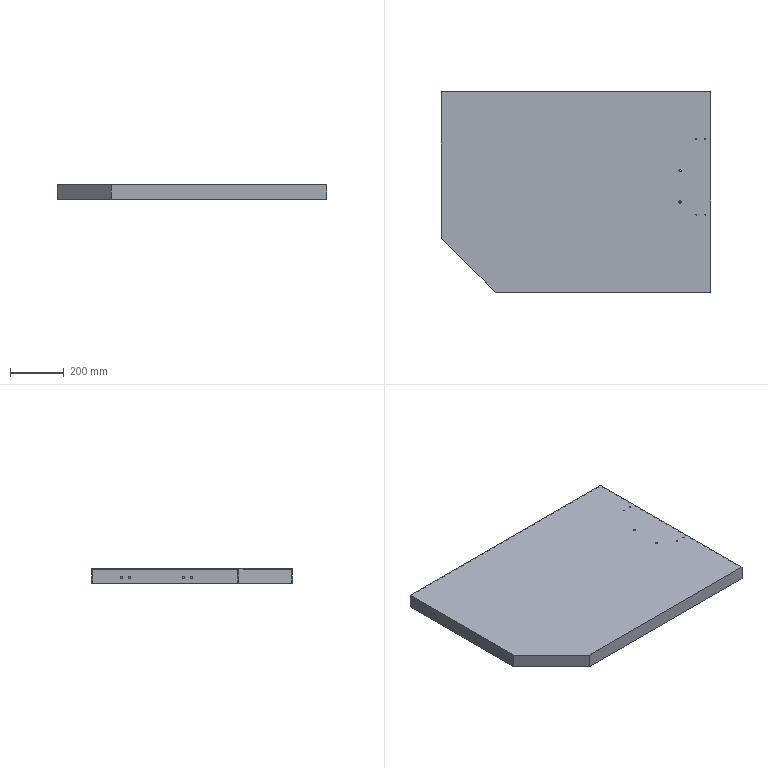Part | SolidWorks | features HoleWzd 2, Cut 1, ExtruThin 1, ICE 1 | 1 solid | 33 faces | box 1000 x 744 x 53 mm | volume 2674985 mm3 | cylinder 20 | plane 13 | commonest cylinder face diameters 4.2 x8 6.8 x8 8.2 x4
STEP:
#1=CARTESIAN_POINT('',(444.915,-62.,50.));
#2=VERTEX_POINT('',#1);
#3=CARTESIAN_POINT('',(449.115,-62.,50.));
#4=VERTEX_POINT('',#3);
#5=CARTESIAN_POINT('',(447.015,-62.,50.));
#6=DIRECTION('',(0.,0.,1.));
#7=DIRECTION('',(1.,0.,0.));
#8=AXIS2_PLACEMENT_3D('',#5,#6,#7);
#9=CIRCLE('',#8,2.1);
#10=EDGE_CURVE('',#2,#4,#9,.T.);
#11=ORIENTED_EDGE('',*,*,#10,.F.);
#12=CARTESIAN_POINT('',(444.915,-62.,53.));
#13=VERTEX_POINT('',#12);
#14=CARTESIAN_POINT('',(444.915,-62.,53.));
#15=DIRECTION('',(0.,0.,1.));
#16=VECTOR('',#15,1000.);
#17=LINE('',#14,#16);
#18=EDGE_CURVE('',#2,#13,#17,.T.);
#19=ORIENTED_EDGE('',*,*,#18,.T.);
#20=CARTESIAN_POINT('',(449.115,-62.,53.));
#21=VERTEX_POINT('',#20);
#22=CARTESIAN_POINT('',(447.015,-62.,53.));
#23=DIRECTION('',(0.,0.,1.));
#24=DIRECTION('',(1.,0.,0.));
#25=AXIS2_PLACEMENT_3D('',#22,#23,#24);
#26=CIRCLE('',#25,2.1);
#27=EDGE_CURVE('',#13,#21,#26,.T.);
#28=ORIENTED_EDGE('',*,*,#27,.T.);
#29=CARTESIAN_POINT('',(449.115,-62.,53.));
#30=DIRECTION('',(0.,0.,1.));
#31=VECTOR('',#30,1000.);
#32=LINE('',#29,#31);
#33=EDGE_CURVE('',#4,#21,#32,.T.);
#34=ORIENTED_EDGE('',*,*,#33,.F.);
#35=EDGE_LOOP('',(#11,#19,#28,#34));
#36=FACE_OUTER_BOUND('',#35,.T.);
#37=CARTESIAN_POINT('',(447.015,-62.,53.));
#38=DIRECTION('',(0.,0.,1.));
#39=DIRECTION('',(1.,0.,0.));
#40=AXIS2_PLACEMENT_3D('',#37,#38,#39);
#41=CYLINDRICAL_SURFACE('',#40,2.1);
#42=ADVANCED_FACE('',(#36),#41,.F.);
#43=CARTESIAN_POINT('',(478.415,-62.,50.));
#44=VERTEX_POINT('',#43);
#45=CARTESIAN_POINT('',(482.615,-62.,50.));
#46=VERTEX_POINT('',#45);
#47=CARTESIAN_POINT('',(480.515,-62.,50.));
#48=DIRECTION('',(0.,0.,1.));
#49=DIRECTION('',(1.,0.,0.));
#50=AXIS2_PLACEMENT_3D('',#47,#48,#49);
#51=CIRCLE('',#50,2.1);
#52=EDGE_CURVE('',#44,#46,#51,.T.);
#53=ORIENTED_EDGE('',*,*,#52,.F.);
#54=CARTESIAN_POINT('',(478.415,-62.,53.));
#55=VERTEX_POINT('',#54);
#56=CARTESIAN_POINT('',(478.415,-62.,53.));
#57=DIRECTION('',(0.,0.,1.));
#58=VECTOR('',#57,1000.);
#59=LINE('',#56,#58);
#60=EDGE_CURVE('',#44,#55,#59,.T.);
#61=ORIENTED_EDGE('',*,*,#60,.T.);
#62=CARTESIAN_POINT('',(482.615,-62.,53.));
#63=VERTEX_POINT('',#62);
#64=CARTESIAN_POINT('',(480.515,-62.,53.));
#65=DIRECTION('',(0.,0.,1.));
#66=DIRECTION('',(1.,0.,0.));
#67=AXIS2_PLACEMENT_3D('',#64,#65,#66);
#68=CIRCLE('',#67,2.1);
#69=EDGE_CURVE('',#55,#63,#68,.T.);
#70=ORIENTED_EDGE('',*,*,#69,.T.);
#71=CARTESIAN_POINT('',(482.615,-62.,53.));
#72=DIRECTION('',(0.,0.,1.));
#73=VECTOR('',#72,1000.);
#74=LINE('',#71,#73);
#75=EDGE_CURVE('',#46,#63,#74,.T.);
#76=ORIENTED_EDGE('',*,*,#75,.F.);
#77=EDGE_LOOP('',(#53,#61,#70,#76));
#78=FACE_OUTER_BOUND('',#77,.T.);
#79=CARTESIAN_POINT('',(480.515,-62.,53.));
#80=DIRECTION('',(0.,0.,1.));
#81=DIRECTION('',(1.,0.,0.));
#82=AXIS2_PLACEMENT_3D('',#79,#80,#81);
#83=CYLINDRICAL_SURFACE('',#82,2.1);
#84=ADVANCED_FACE('',(#78),#83,.F.);
#85=CARTESIAN_POINT('',(444.915,218.,50.));
#86=VERTEX_POINT('',#85);
#87=CARTESIAN_POINT('',(449.115,218.,50.));
#88=VERTEX_POINT('',#87);
#89=CARTESIAN_POINT('',(447.015,218.,50.));
#90=DIRECTION('',(0.,0.,1.));
#91=DIRECTION('',(1.,0.,0.));
#92=AXIS2_PLACEMENT_3D('',#89,#90,#91);
#93=CIRCLE('',#92,2.1);
#94=EDGE_CURVE('',#86,#88,#93,.T.);
#95=ORIENTED_EDGE('',*,*,#94,.F.);
#96=CARTESIAN_POINT('',(444.915,218.,53.));
#97=VERTEX_POINT('',#96);
#98=CARTESIAN_POINT('',(444.915,218.,53.));
#99=DIRECTION('',(0.,0.,1.));
#100=VECTOR('',#99,1000.);
#101=LINE('',#98,#100);
#102=EDGE_CURVE('',#86,#97,#101,.T.);
#103=ORIENTED_EDGE('',*,*,#102,.T.);
#104=CARTESIAN_POINT('',(449.115,218.,53.));
#105=VERTEX_POINT('',#104);
#106=CARTESIAN_POINT('',(447.015,218.,53.));
#107=DIRECTION('',(0.,0.,1.));
#108=DIRECTION('',(1.,0.,0.));
#109=AXIS2_PLACEMENT_3D('',#106,#107,#108);
#110=CIRCLE('',#109,2.1);
#111=EDGE_CURVE('',#97,#105,#110,.T.);
#112=ORIENTED_EDGE('',*,*,#111,.T.);
#113=CARTESIAN_POINT('',(449.115,218.,53.));
#114=DIRECTION('',(0.,0.,1.));
#115=VECTOR('',#114,1000.);
#116=LINE('',#113,#115);
#117=EDGE_CURVE('',#88,#105,#116,.T.);
#118=ORIENTED_EDGE('',*,*,#117,.F.);
#119=EDGE_LOOP('',(#95,#103,#112,#118));
#120=FACE_OUTER_BOUND('',#119,.T.);
#121=CARTESIAN_POINT('',(447.015,218.,53.));
#122=DIRECTION('',(0.,0.,1.));
#123=DIRECTION('',(1.,0.,0.));
#124=AXIS2_PLACEMENT_3D('',#121,#122,#123);
#125=CYLINDRICAL_SURFACE('',#124,2.1);
#126=ADVANCED_FACE('',(#120),#125,.F.);
#127=CARTESIAN_POINT('',(478.415,218.,50.));
#128=VERTEX_POINT('',#127);
#129=CARTESIAN_POINT('',(482.615,218.,50.));
#130=VERTEX_POINT('',#129);
#131=CARTESIAN_POINT('',(480.515,218.,50.));
#132=DIRECTION('',(0.,0.,1.));
#133=DIRECTION('',(1.,0.,0.));
#134=AXIS2_PLACEMENT_3D('',#131,#132,#133);
#135=CIRCLE('',#134,2.1);
#136=EDGE_CURVE('',#128,#130,#135,.T.);
#137=ORIENTED_EDGE('',*,*,#136,.F.);
#138=CARTESIAN_POINT('',(478.415,218.,53.));
#139=VERTEX_POINT('',#138);
#140=CARTESIAN_POINT('',(478.415,218.,53.));
#141=DIRECTION('',(0.,0.,1.));
#142=VECTOR('',#141,1000.);
#143=LINE('',#140,#142);
#144=EDGE_CURVE('',#128,#139,#143,.T.);
#145=ORIENTED_EDGE('',*,*,#144,.T.);
#146=CARTESIAN_POINT('',(482.615,218.,53.));
#147=VERTEX_POINT('',#146);
#148=CARTESIAN_POINT('',(480.515,218.,53.));
#149=DIRECTION('',(0.,0.,1.));
#150=DIRECTION('',(1.,0.,0.));
#151=AXIS2_PLACEMENT_3D('',#148,#149,#150);
#152=CIRCLE('',#151,2.1);
#153=EDGE_CURVE('',#139,#147,#152,.T.);
#154=ORIENTED_EDGE('',*,*,#153,.T.);
#155=CARTESIAN_POINT('',(482.615,218.,53.));
#156=DIRECTION('',(0.,0.,1.));
#157=VECTOR('',#156,1000.);
#158=LINE('',#155,#157);
#159=EDGE_CURVE('',#130,#147,#158,.T.);
#160=ORIENTED_EDGE('',*,*,#159,.F.);
#161=EDGE_LOOP('',(#137,#145,#154,#160));
#162=FACE_OUTER_BOUND('',#161,.T.);
#163=CARTESIAN_POINT('',(480.515,218.,53.));
#164=DIRECTION('',(0.,0.,1.));
#165=DIRECTION('',(1.,0.,0.));
#166=AXIS2_PLACEMENT_3D('',#163,#164,#165);
#167=CYLINDRICAL_SURFACE('',#166,2.1);
#168=ADVANCED_FACE('',(#162),#167,.F.);
#169=CARTESIAN_POINT('',(-497.,284.,24.4));
#170=VERTEX_POINT('',#169);
#171=CARTESIAN_POINT('',(-497.,284.,17.6));
#172=VERTEX_POINT('',#171);
#173=CARTESIAN_POINT('',(-497.,284.,21.));
#174=DIRECTION('',(1.,0.,0.));
#175=DIRECTION('',(0.,1.,0.));
#176=AXIS2_PLACEMENT_3D('',#173,#174,#175);
#177=CIRCLE('',#176,3.4);
#178=EDGE_CURVE('',#170,#172,#177,.T.);
#179=ORIENTED_EDGE('',*,*,#178,.T.);
#180=CARTESIAN_POINT('',(-500.,284.,17.6));
#181=VERTEX_POINT('',#180);
#182=CARTESIAN_POINT('',(-500.,284.,17.6));
#183=DIRECTION('',(-1.,0.,0.));
#184=VECTOR('',#183,1000.);
#185=LINE('',#182,#184);
#186=EDGE_CURVE('',#172,#181,#185,.T.);
#187=ORIENTED_EDGE('',*,*,#186,.T.);
#188=CARTESIAN_POINT('',(-500.,284.,24.4));
#189=VERTEX_POINT('',#188);
#190=CARTESIAN_POINT('',(-500.,284.,21.));
#191=DIRECTION('',(-1.,0.,0.));
#192=DIRECTION('',(0.,0.,1.));
#193=AXIS2_PLACEMENT_3D('',#190,#191,#192);
#194=CIRCLE('',#193,3.4);
#195=EDGE_CURVE('',#181,#189,#194,.T.);
#196=ORIENTED_EDGE('',*,*,#195,.T.);
#197=CARTESIAN_POINT('',(-500.,284.,24.4));
#198=DIRECTION('',(-1.,0.,0.));
#199=VECTOR('',#198,1000.);
#200=LINE('',#197,#199);
#201=EDGE_CURVE('',#170,#189,#200,.T.);
#202=ORIENTED_EDGE('',*,*,#201,.F.);
#203=EDGE_LOOP('',(#179,#187,#196,#202));
#204=FACE_OUTER_BOUND('',#203,.T.);
#205=CARTESIAN_POINT('',(-500.,284.,21.));
#206=DIRECTION('',(-1.,0.,0.));
#207=DIRECTION('',(0.,0.,1.));
#208=AXIS2_PLACEMENT_3D('',#205,#206,#207);
#209=CYLINDRICAL_SURFACE('',#208,3.4);
#210=ADVANCED_FACE('',(#204),#209,.F.);
#211=CARTESIAN_POINT('',(-497.,254.,24.4));
#212=VERTEX_POINT('',#211);
#213=CARTESIAN_POINT('',(-497.,254.,17.6));
#214=VERTEX_POINT('',#213);
#215=CARTESIAN_POINT('',(-497.,254.,21.));
#216=DIRECTION('',(1.,0.,0.));
#217=DIRECTION('',(0.,1.,0.));
#218=AXIS2_PLACEMENT_3D('',#215,#216,#217);
#219=CIRCLE('',#218,3.4);
#220=EDGE_CURVE('',#212,#214,#219,.T.);
#221=ORIENTED_EDGE('',*,*,#220,.T.);
#222=CARTESIAN_POINT('',(-500.,254.,17.6));
#223=VERTEX_POINT('',#222);
#224=CARTESIAN_POINT('',(-500.,254.,17.6));
#225=DIRECTION('',(-1.,0.,0.));
#226=VECTOR('',#225,1000.);
#227=LINE('',#224,#226);
#228=EDGE_CURVE('',#214,#223,#227,.T.);
#229=ORIENTED_EDGE('',*,*,#228,.T.);
#230=CARTESIAN_POINT('',(-500.,254.,24.4));
#231=VERTEX_POINT('',#230);
#232=CARTESIAN_POINT('',(-500.,254.,21.));
#233=DIRECTION('',(-1.,0.,0.));
#234=DIRECTION('',(0.,0.,1.));
#235=AXIS2_PLACEMENT_3D('',#232,#233,#234);
#236=CIRCLE('',#235,3.4);
#237=EDGE_CURVE('',#223,#231,#236,.T.);
#238=ORIENTED_EDGE('',*,*,#237,.T.);
#239=CARTESIAN_POINT('',(-500.,254.,24.4));
#240=DIRECTION('',(-1.,0.,0.));
#241=VECTOR('',#240,1000.);
#242=LINE('',#239,#241);
#243=EDGE_CURVE('',#212,#231,#242,.T.);
#244=ORIENTED_EDGE('',*,*,#243,.F.);
#245=EDGE_LOOP('',(#221,#229,#238,#244));
#246=FACE_OUTER_BOUND('',#245,.T.);
#247=CARTESIAN_POINT('',(-500.,254.,21.));
#248=DIRECTION('',(-1.,0.,0.));
#249=DIRECTION('',(0.,0.,1.));
#250=AXIS2_PLACEMENT_3D('',#247,#248,#249);
#251=CYLINDRICAL_SURFACE('',#250,3.4);
#252=ADVANCED_FACE('',(#246),#251,.F.);
#253=CARTESIAN_POINT('',(-497.,54.,24.4));
#254=VERTEX_POINT('',#253);
#255=CARTESIAN_POINT('',(-497.,54.,17.6));
#256=VERTEX_POINT('',#255);
#257=CARTESIAN_POINT('',(-497.,54.,21.));
#258=DIRECTION('',(1.,0.,0.));
#259=DIRECTION('',(0.,1.,0.));
#260=AXIS2_PLACEMENT_3D('',#257,#258,#259);
#261=CIRCLE('',#260,3.4);
#262=EDGE_CURVE('',#254,#256,#261,.T.);
#263=ORIENTED_EDGE('',*,*,#262,.T.);
#264=CARTESIAN_POINT('',(-500.,54.,17.6));
#265=VERTEX_POINT('',#264);
#266=CARTESIAN_POINT('',(-500.,54.,17.6));
#267=DIRECTION('',(-1.,0.,0.));
#268=VECTOR('',#267,1000.);
#269=LINE('',#266,#268);
#270=EDGE_CURVE('',#256,#265,#269,.T.);
#271=ORIENTED_EDGE('',*,*,#270,.T.);
#272=CARTESIAN_POINT('',(-500.,54.,24.4));
#273=VERTEX_POINT('',#272);
#274=CARTESIAN_POINT('',(-500.,54.,21.));
#275=DIRECTION('',(-1.,0.,0.));
#276=DIRECTION('',(0.,0.,1.));
#277=AXIS2_PLACEMENT_3D('',#274,#275,#276);
#278=CIRCLE('',#277,3.4);
#279=EDGE_CURVE('',#265,#273,#278,.T.);
#280=ORIENTED_EDGE('',*,*,#279,.T.);
#281=CARTESIAN_POINT('',(-500.,54.,24.4));
#282=DIRECTION('',(-1.,0.,0.));
#283=VECTOR('',#282,1000.);
#284=LINE('',#281,#283);
#285=EDGE_CURVE('',#254,#273,#284,.T.);
#286=ORIENTED_EDGE('',*,*,#285,.F.);
#287=EDGE_LOOP('',(#263,#271,#280,#286));
#288=FACE_OUTER_BOUND('',#287,.T.);
#289=CARTESIAN_POINT('',(-500.,54.,21.));
#290=DIRECTION('',(-1.,0.,0.));
#291=DIRECTION('',(0.,0.,1.));
#292=AXIS2_PLACEMENT_3D('',#289,#290,#291);
#293=CYLINDRICAL_SURFACE('',#292,3.4);
#294=ADVANCED_FACE('',(#288),#293,.F.);
#295=CARTESIAN_POINT('',(-497.,24.,24.4));
#296=VERTEX_POINT('',#295);
#297=CARTESIAN_POINT('',(-497.,24.,17.6));
#298=VERTEX_POINT('',#297);
#299=CARTESIAN_POINT('',(-497.,24.,21.));
#300=DIRECTION('',(1.,0.,0.));
#301=DIRECTION('',(0.,1.,0.));
#302=AXIS2_PLACEMENT_3D('',#299,#300,#301);
#303=CIRCLE('',#302,3.4);
#304=EDGE_CURVE('',#296,#298,#303,.T.);
#305=ORIENTED_EDGE('',*,*,#304,.T.);
#306=CARTESIAN_POINT('',(-500.,24.,17.6));
#307=VERTEX_POINT('',#306);
#308=CARTESIAN_POINT('',(-500.,24.,17.6));
#309=DIRECTION('',(-1.,0.,0.));
#310=VECTOR('',#309,1000.);
#311=LINE('',#308,#310);
#312=EDGE_CURVE('',#298,#307,#311,.T.);
#313=ORIENTED_EDGE('',*,*,#312,.T.);
#314=CARTESIAN_POINT('',(-500.,24.,24.4));
#315=VERTEX_POINT('',#314);
#316=CARTESIAN_POINT('',(-500.,24.,21.));
#317=DIRECTION('',(-1.,0.,0.));
#318=DIRECTION('',(0.,0.,1.));
#319=AXIS2_PLACEMENT_3D('',#316,#317,#318);
#320=CIRCLE('',#319,3.4);
#321=EDGE_CURVE('',#307,#315,#320,.T.);
#322=ORIENTED_EDGE('',*,*,#321,.T.);
#323=CARTESIAN_POINT('',(-500.,24.,24.4));
#324=DIRECTION('',(-1.,0.,0.));
#325=VECTOR('',#324,1000.);
#326=LINE('',#323,#325);
#327=EDGE_CURVE('',#296,#315,#326,.T.);
#328=ORIENTED_EDGE('',*,*,#327,.F.);
#329=EDGE_LOOP('',(#305,#313,#322,#328));
#330=FACE_OUTER_BOUND('',#329,.T.);
#331=CARTESIAN_POINT('',(-500.,24.,21.));
#332=DIRECTION('',(-1.,0.,0.));
#333=DIRECTION('',(0.,0.,1.));
#334=AXIS2_PLACEMENT_3D('',#331,#332,#333);
#335=CYLINDRICAL_SURFACE('',#334,3.4);
#336=ADVANCED_FACE('',(#330),#335,.F.);
#337=CARTESIAN_POINT('',(390.6,101.25,50.));
#338=VERTEX_POINT('',#337);
#339=CARTESIAN_POINT('',(382.4,101.25,50.));
#340=VERTEX_POINT('',#339);
#341=CARTESIAN_POINT('',(386.5,101.25,50.));
#342=DIRECTION('',(0.,0.,-1.));
#343=DIRECTION('',(1.,0.,0.));
#344=AXIS2_PLACEMENT_3D('',#341,#342,#343);
#345=CIRCLE('',#344,4.1);
#346=EDGE_CURVE('',#338,#340,#345,.T.);
#347=ORIENTED_EDGE('',*,*,#346,.T.);
#348=CARTESIAN_POINT('',(382.4,101.25,53.));
#349=VERTEX_POINT('',#348);
#350=CARTESIAN_POINT('',(382.4,101.25,-0.001));
#351=DIRECTION('',(0.,0.,1.));
#352=VECTOR('',#351,1000.);
#353=LINE('',#350,#352);
#354=EDGE_CURVE('',#340,#349,#353,.T.);
#355=ORIENTED_EDGE('',*,*,#354,.T.);
#356=CARTESIAN_POINT('',(390.6,101.25,53.));
#357=VERTEX_POINT('',#356);
#358=CARTESIAN_POINT('',(386.5,101.25,53.));
#359=DIRECTION('',(0.,0.,1.));
#360=DIRECTION('',(1.,0.,0.));
#361=AXIS2_PLACEMENT_3D('',#358,#359,#360);
#362=CIRCLE('',#361,4.1);
#363=EDGE_CURVE('',#349,#357,#362,.T.);
#364=ORIENTED_EDGE('',*,*,#363,.T.);
#365=CARTESIAN_POINT('',(390.6,101.25,-0.001));
#366=DIRECTION('',(0.,0.,1.));
#367=VECTOR('',#366,1000.);
#368=LINE('',#365,#367);
#369=EDGE_CURVE('',#338,#357,#368,.T.);
#370=ORIENTED_EDGE('',*,*,#369,.F.);
#371=EDGE_LOOP('',(#347,#355,#364,#370));
#372=FACE_OUTER_BOUND('',#371,.T.);
#373=CARTESIAN_POINT('',(386.5,101.25,-0.001));
#374=DIRECTION('',(0.,0.,1.));
#375=DIRECTION('',(1.,0.,0.));
#376=AXIS2_PLACEMENT_3D('',#373,#374,#375);
#377=CYLINDRICAL_SURFACE('',#376,4.1);
#378=ADVANCED_FACE('',(#372),#377,.F.);
#379=CARTESIAN_POINT('',(390.6,-15.25,50.));
#380=VERTEX_POINT('',#379);
#381=CARTESIAN_POINT('',(382.4,-15.25,50.));
#382=VERTEX_POINT('',#381);
#383=CARTESIAN_POINT('',(386.5,-15.25,50.));
#384=DIRECTION('',(0.,0.,-1.));
#385=DIRECTION('',(1.,0.,0.));
#386=AXIS2_PLACEMENT_3D('',#383,#384,#385);
#387=CIRCLE('',#386,4.1);
#388=EDGE_CURVE('',#380,#382,#387,.T.);
#389=ORIENTED_EDGE('',*,*,#388,.T.);
#390=CARTESIAN_POINT('',(382.4,-15.25,53.));
#391=VERTEX_POINT('',#390);
#392=CARTESIAN_POINT('',(382.4,-15.25,-0.001));
#393=DIRECTION('',(0.,0.,1.));
#394=VECTOR('',#393,1000.);
#395=LINE('',#392,#394);
#396=EDGE_CURVE('',#382,#391,#395,.T.);
#397=ORIENTED_EDGE('',*,*,#396,.T.);
#398=CARTESIAN_POINT('',(390.6,-15.25,53.));
#399=VERTEX_POINT('',#398);
#400=CARTESIAN_POINT('',(386.5,-15.25,53.));
#401=DIRECTION('',(0.,0.,1.));
#402=DIRECTION('',(1.,0.,0.));
#403=AXIS2_PLACEMENT_3D('',#400,#401,#402);
#404=CIRCLE('',#403,4.1);
#405=EDGE_CURVE('',#391,#399,#404,.T.);
#406=ORIENTED_EDGE('',*,*,#405,.T.);
#407=CARTESIAN_POINT('',(390.6,-15.25,-0.001));
#408=DIRECTION('',(0.,0.,1.));
#409=VECTOR('',#408,1000.);
#410=LINE('',#407,#409);
#411=EDGE_CURVE('',#380,#399,#410,.T.);
#412=ORIENTED_EDGE('',*,*,#411,.F.);
#413=EDGE_LOOP('',(#389,#397,#406,#412));
#414=FACE_OUTER_BOUND('',#413,.T.);
#415=CARTESIAN_POINT('',(386.5,-15.25,-0.001));
#416=DIRECTION('',(0.,0.,1.));
#417=DIRECTION('',(1.,0.,0.));
#418=AXIS2_PLACEMENT_3D('',#415,#416,#417);
#419=CYLINDRICAL_SURFACE('',#418,4.1);
#420=ADVANCED_FACE('',(#414),#419,.F.);
#421=CARTESIAN_POINT('',(-500.,-150.,0.));
#422=VERTEX_POINT('',#421);
#423=CARTESIAN_POINT('',(-300.,-350.,0.));
#424=VERTEX_POINT('',#423);
#425=CARTESIAN_POINT('',(-500.,-150.,0.));
#426=DIRECTION('',(0.7071,-0.7071,0.));
#427=VECTOR('',#426,1000.);
#428=LINE('',#425,#427);
#429=EDGE_CURVE('',#422,#424,#428,.T.);
#430=ORIENTED_EDGE('',*,*,#429,.F.);
#431=CARTESIAN_POINT('',(-500.,394.,0.));
#432=VERTEX_POINT('',#431);
#433=CARTESIAN_POINT('',(-500.,394.,0.));
#434=DIRECTION('',(0.,-1.,0.));
#435=VECTOR('',#434,1000.);
#436=LINE('',#433,#435);
#437=EDGE_CURVE('',#432,#422,#436,.T.);
#438=ORIENTED_EDGE('',*,*,#437,.F.);
#439=CARTESIAN_POINT('',(500.,394.,0.));
#440=VERTEX_POINT('',#439);
#441=CARTESIAN_POINT('',(500.,394.,0.));
#442=DIRECTION('',(-1.,0.,0.));
#443=VECTOR('',#442,1000.);
#444=LINE('',#441,#443);
#445=EDGE_CURVE('',#440,#432,#444,.T.);
#446=ORIENTED_EDGE('',*,*,#445,.F.);
#447=CARTESIAN_POINT('',(500.,-350.,0.));
#448=VERTEX_POINT('',#447);
#449=CARTESIAN_POINT('',(500.,-350.,0.));
#450=DIRECTION('',(0.,1.,0.));
#451=VECTOR('',#450,1000.);
#452=LINE('',#449,#451);
#453=EDGE_CURVE('',#448,#440,#452,.T.);
#454=ORIENTED_EDGE('',*,*,#453,.F.);
#455=CARTESIAN_POINT('',(-300.,-350.,0.));
#456=DIRECTION('',(1.,0.,0.));
#457=VECTOR('',#456,1000.);
#458=LINE('',#455,#457);
#459=EDGE_CURVE('',#424,#448,#458,.T.);
#460=ORIENTED_EDGE('',*,*,#459,.F.);
#461=EDGE_LOOP('',(#430,#438,#446,#454,#460));
#462=FACE_OUTER_BOUND('',#461,.T.);
#463=CARTESIAN_POINT('',(-497.,-148.757,0.));
#464=VERTEX_POINT('',#463);
#465=CARTESIAN_POINT('',(-298.757,-347.,0.));
#466=VERTEX_POINT('',#465);
#467=CARTESIAN_POINT('',(-497.879,-147.879,0.));
#468=DIRECTION('',(0.7071,-0.7071,0.));
#469=VECTOR('',#468,1000.);
#470=LINE('',#467,#469);
#471=EDGE_CURVE('',#464,#466,#470,.T.);
#472=ORIENTED_EDGE('',*,*,#471,.T.);
#473=CARTESIAN_POINT('',(497.,-347.,0.));
#474=VERTEX_POINT('',#473);
#475=CARTESIAN_POINT('',(-300.,-347.,0.));
#476=DIRECTION('',(1.,0.,0.));
#477=VECTOR('',#476,1000.);
#478=LINE('',#475,#477);
#479=EDGE_CURVE('',#466,#474,#478,.T.);
#480=ORIENTED_EDGE('',*,*,#479,.T.);
#481=CARTESIAN_POINT('',(497.,391.,0.));
#482=VERTEX_POINT('',#481);
#483=CARTESIAN_POINT('',(497.,-350.,0.));
#484=DIRECTION('',(0.,1.,0.));
#485=VECTOR('',#484,1000.);
#486=LINE('',#483,#485);
#487=EDGE_CURVE('',#474,#482,#486,.T.);
#488=ORIENTED_EDGE('',*,*,#487,.T.);
#489=CARTESIAN_POINT('',(-497.,391.,0.));
#490=VERTEX_POINT('',#489);
#491=CARTESIAN_POINT('',(500.,391.,0.));
#492=DIRECTION('',(-1.,0.,0.));
#493=VECTOR('',#492,1000.);
#494=LINE('',#491,#493);
#495=EDGE_CURVE('',#482,#490,#494,.T.);
#496=ORIENTED_EDGE('',*,*,#495,.T.);
#497=CARTESIAN_POINT('',(-497.,394.,0.));
#498=DIRECTION('',(0.,-1.,0.));
#499=VECTOR('',#498,1000.);
#500=LINE('',#497,#499);
#501=EDGE_CURVE('',#490,#464,#500,.T.);
#502=ORIENTED_EDGE('',*,*,#501,.T.);
#503=EDGE_LOOP('',(#472,#480,#488,#496,#502));
#504=FACE_BOUND('',#503,.T.);
#505=CARTESIAN_POINT('',(0.,0.,0.));
#506=DIRECTION('',(0.,0.,1.));
#507=DIRECTION('',(1.,0.,0.));
#508=AXIS2_PLACEMENT_3D('',#505,#506,#507);
#509=PLANE('',#508);
#510=ADVANCED_FACE('',(#462,#504),#509,.F.);
#511=ORIENTED_EDGE('',*,*,#429,.T.);
#512=CARTESIAN_POINT('',(-300.,-350.,53.));
#513=VERTEX_POINT('',#512);
#514=CARTESIAN_POINT('',(-300.,-350.,50.));
#515=DIRECTION('',(0.,0.,-1.));
#516=VECTOR('',#515,1000.);
#517=LINE('',#514,#516);
#518=EDGE_CURVE('',#513,#424,#517,.T.);
#519=ORIENTED_EDGE('',*,*,#518,.F.);
#520=CARTESIAN_POINT('',(-500.,-150.,53.));
#521=VERTEX_POINT('',#520);
#522=CARTESIAN_POINT('',(-500.,-150.,53.));
#523=DIRECTION('',(0.7071,-0.7071,0.));
#524=VECTOR('',#523,1000.);
#525=LINE('',#522,#524);
#526=EDGE_CURVE('',#521,#513,#525,.T.);
#527=ORIENTED_EDGE('',*,*,#526,.F.);
#528=CARTESIAN_POINT('',(-500.,-150.,50.));
#529=DIRECTION('',(0.,0.,-1.));
#530=VECTOR('',#529,1000.);
#531=LINE('',#528,#530);
#532=EDGE_CURVE('',#521,#422,#531,.T.);
#533=ORIENTED_EDGE('',*,*,#532,.T.);
#534=EDGE_LOOP('',(#511,#519,#527,#533));
#535=FACE_OUTER_BOUND('',#534,.T.);
#536=CARTESIAN_POINT('',(-500.,-150.,50.));
#537=DIRECTION('',(0.7071,0.7071,0.));
#538=DIRECTION('',(-0.7071,0.7071,0.));
#539=AXIS2_PLACEMENT_3D('',#536,#537,#538);
#540=PLANE('',#539);
#541=ADVANCED_FACE('',(#535),#540,.F.);
#542=ORIENTED_EDGE('',*,*,#459,.T.);
#543=CARTESIAN_POINT('',(500.,-350.,53.));
#544=VERTEX_POINT('',#543);
#545=CARTESIAN_POINT('',(500.,-350.,50.));
#546=DIRECTION('',(0.,0.,-1.));
#547=VECTOR('',#546,1000.);
#548=LINE('',#545,#547);
#549=EDGE_CURVE('',#544,#448,#548,.T.);
#550=ORIENTED_EDGE('',*,*,#549,.F.);
#551=CARTESIAN_POINT('',(-300.,-350.,53.));
#552=DIRECTION('',(1.,0.,0.));
#553=VECTOR('',#552,1000.);
#554=LINE('',#551,#553);
#555=EDGE_CURVE('',#513,#544,#554,.T.);
#556=ORIENTED_EDGE('',*,*,#555,.F.);
#557=ORIENTED_EDGE('',*,*,#518,.T.);
#558=EDGE_LOOP('',(#542,#550,#556,#557));
#559=FACE_OUTER_BOUND('',#558,.T.);
#560=CARTESIAN_POINT('',(-300.,-350.,50.));
#561=DIRECTION('',(0.,1.,0.));
#562=DIRECTION('',(0.,0.,1.));
#563=AXIS2_PLACEMENT_3D('',#560,#561,#562);
#564=PLANE('',#563);
#565=ADVANCED_FACE('',(#559),#564,.F.);
#566=ORIENTED_EDGE('',*,*,#453,.T.);
#567=CARTESIAN_POINT('',(500.,394.,53.));
#568=VERTEX_POINT('',#567);
#569=CARTESIAN_POINT('',(500.,394.,50.));
#570=DIRECTION('',(0.,0.,-1.));
#571=VECTOR('',#570,1000.);
#572=LINE('',#569,#571);
#573=EDGE_CURVE('',#568,#440,#572,.T.);
#574=ORIENTED_EDGE('',*,*,#573,.F.);
#575=CARTESIAN_POINT('',(500.,-350.,53.));
#576=DIRECTION('',(0.,1.,0.));
#577=VECTOR('',#576,1000.);
#578=LINE('',#575,#577);
#579=EDGE_CURVE('',#544,#568,#578,.T.);
#580=ORIENTED_EDGE('',*,*,#579,.F.);
#581=ORIENTED_EDGE('',*,*,#549,.T.);
#582=EDGE_LOOP('',(#566,#574,#580,#581));
#583=FACE_OUTER_BOUND('',#582,.T.);
#584=CARTESIAN_POINT('',(500.,-350.,50.));
#585=DIRECTION('',(-1.,0.,0.));
#586=DIRECTION('',(0.,0.,1.));
#587=AXIS2_PLACEMENT_3D('',#584,#585,#586);
#588=PLANE('',#587);
#589=ADVANCED_FACE('',(#583),#588,.F.);
#590=ORIENTED_EDGE('',*,*,#445,.T.);
#591=CARTESIAN_POINT('',(-500.,394.,53.));
#592=VERTEX_POINT('',#591);
#593=CARTESIAN_POINT('',(-500.,394.,50.));
#594=DIRECTION('',(0.,0.,-1.));
#595=VECTOR('',#594,1000.);
#596=LINE('',#593,#595);
#597=EDGE_CURVE('',#592,#432,#596,.T.);
#598=ORIENTED_EDGE('',*,*,#597,.F.);
#599=CARTESIAN_POINT('',(500.,394.,53.));
#600=DIRECTION('',(-1.,0.,0.));
#601=VECTOR('',#600,1000.);
#602=LINE('',#599,#601);
#603=EDGE_CURVE('',#568,#592,#602,.T.);
#604=ORIENTED_EDGE('',*,*,#603,.F.);
#605=ORIENTED_EDGE('',*,*,#573,.T.);
#606=EDGE_LOOP('',(#590,#598,#604,#605));
#607=FACE_OUTER_BOUND('',#606,.T.);
#608=CARTESIAN_POINT('',(500.,394.,50.));
#609=DIRECTION('',(0.,-1.,0.));
#610=DIRECTION('',(1.,0.,0.));
#611=AXIS2_PLACEMENT_3D('',#608,#609,#610);
#612=PLANE('',#611);
#613=ADVANCED_FACE('',(#607),#612,.F.);
#614=CARTESIAN_POINT('',(-500.,284.,21.));
#615=DIRECTION('',(-1.,0.,0.));
#616=DIRECTION('',(0.,0.,1.));
#617=AXIS2_PLACEMENT_3D('',#614,#615,#616);
#618=CIRCLE('',#617,3.4);
#619=EDGE_CURVE('',#189,#181,#618,.T.);
#620=ORIENTED_EDGE('',*,*,#619,.F.);
#621=ORIENTED_EDGE('',*,*,#195,.F.);
#622=EDGE_LOOP('',(#620,#621));
#623=FACE_BOUND('',#622,.T.);
#624=CARTESIAN_POINT('',(-500.,254.,21.));
#625=DIRECTION('',(-1.,0.,0.));
#626=DIRECTION('',(0.,0.,1.));
#627=AXIS2_PLACEMENT_3D('',#624,#625,#626);
#628=CIRCLE('',#627,3.4);
#629=EDGE_CURVE('',#231,#223,#628,.T.);
#630=ORIENTED_EDGE('',*,*,#629,.F.);
#631=ORIENTED_EDGE('',*,*,#237,.F.);
#632=EDGE_LOOP('',(#630,#631));
#633=FACE_BOUND('',#632,.T.);
#634=CARTESIAN_POINT('',(-500.,54.,21.));
#635=DIRECTION('',(-1.,0.,0.));
#636=DIRECTION('',(0.,0.,1.));
#637=AXIS2_PLACEMENT_3D('',#634,#635,#636);
#638=CIRCLE('',#637,3.4);
#639=EDGE_CURVE('',#273,#265,#638,.T.);
#640=ORIENTED_EDGE('',*,*,#639,.F.);
#641=ORIENTED_EDGE('',*,*,#279,.F.);
#642=EDGE_LOOP('',(#640,#641));
#643=FACE_BOUND('',#642,.T.);
#644=CARTESIAN_POINT('',(-500.,24.,21.));
#645=DIRECTION('',(-1.,0.,0.));
#646=DIRECTION('',(0.,0.,1.));
#647=AXIS2_PLACEMENT_3D('',#644,#645,#646);
#648=CIRCLE('',#647,3.4);
#649=EDGE_CURVE('',#315,#307,#648,.T.);
#650=ORIENTED_EDGE('',*,*,#649,.F.);
#651=ORIENTED_EDGE('',*,*,#321,.F.);
#652=EDGE_LOOP('',(#650,#651));
#653=FACE_BOUND('',#652,.T.);
#654=ORIENTED_EDGE('',*,*,#437,.T.);
#655=ORIENTED_EDGE('',*,*,#532,.F.);
#656=CARTESIAN_POINT('',(-500.,394.,53.));
#657=DIRECTION('',(0.,-1.,0.));
#658=VECTOR('',#657,1000.);
#659=LINE('',#656,#658);
#660=EDGE_CURVE('',#592,#521,#659,.T.);
#661=ORIENTED_EDGE('',*,*,#660,.F.);
#662=ORIENTED_EDGE('',*,*,#597,.T.);
#663=EDGE_LOOP('',(#654,#655,#661,#662));
#664=FACE_OUTER_BOUND('',#663,.T.);
#665=CARTESIAN_POINT('',(-500.,394.,50.));
#666=DIRECTION('',(1.,0.,0.));
#667=DIRECTION('',(0.,1.,0.));
#668=AXIS2_PLACEMENT_3D('',#665,#666,#667);
#669=PLANE('',#668);
#670=ADVANCED_FACE('',(#623,#633,#643,#653,#664),#669,.F.);
#671=ORIENTED_EDGE('',*,*,#471,.F.);
#672=CARTESIAN_POINT('',(-497.,-148.757,50.));
#673=VERTEX_POINT('',#672);
#674=CARTESIAN_POINT('',(-497.,-148.757,50.));
#675=DIRECTION('',(0.,0.,-1.));
#676=VECTOR('',#675,1000.);
#677=LINE('',#674,#676);
#678=EDGE_CURVE('',#673,#464,#677,.T.);
#679=ORIENTED_EDGE('',*,*,#678,.F.);
#680=CARTESIAN_POINT('',(-298.757,-347.,50.));
#681=VERTEX_POINT('',#680);
#682=CARTESIAN_POINT('',(-497.879,-147.879,50.));
#683=DIRECTION('',(0.7071,-0.7071,0.));
#684=VECTOR('',#683,1000.);
#685=LINE('',#682,#684);
#686=EDGE_CURVE('',#673,#681,#685,.T.);
#687=ORIENTED_EDGE('',*,*,#686,.T.);
#688=CARTESIAN_POINT('',(-298.757,-347.,50.));
#689=DIRECTION('',(0.,0.,-1.));
#690=VECTOR('',#689,1000.);
#691=LINE('',#688,#690);
#692=EDGE_CURVE('',#681,#466,#691,.T.);
#693=ORIENTED_EDGE('',*,*,#692,.T.);
#694=EDGE_LOOP('',(#671,#679,#687,#693));
#695=FACE_OUTER_BOUND('',#694,.T.);
#696=CARTESIAN_POINT('',(-497.879,-147.879,50.));
#697=DIRECTION('',(0.7071,0.7071,0.));
#698=DIRECTION('',(-0.7071,0.7071,0.));
#699=AXIS2_PLACEMENT_3D('',#696,#697,#698);
#700=PLANE('',#699);
#701=ADVANCED_FACE('',(#695),#700,.T.);
#702=ORIENTED_EDGE('',*,*,#479,.F.);
#703=ORIENTED_EDGE('',*,*,#692,.F.);
#704=CARTESIAN_POINT('',(497.,-347.,50.));
#705=VERTEX_POINT('',#704);
#706=CARTESIAN_POINT('',(-300.,-347.,50.));
#707=DIRECTION('',(1.,0.,0.));
#708=VECTOR('',#707,1000.);
#709=LINE('',#706,#708);
#710=EDGE_CURVE('',#681,#705,#709,.T.);
#711=ORIENTED_EDGE('',*,*,#710,.T.);
#712=CARTESIAN_POINT('',(497.,-347.,50.));
#713=DIRECTION('',(0.,0.,-1.));
#714=VECTOR('',#713,1000.);
#715=LINE('',#712,#714);
#716=EDGE_CURVE('',#705,#474,#715,.T.);
#717=ORIENTED_EDGE('',*,*,#716,.T.);
#718=EDGE_LOOP('',(#702,#703,#711,#717));
#719=FACE_OUTER_BOUND('',#718,.T.);
#720=CARTESIAN_POINT('',(-300.,-347.,50.));
#721=DIRECTION('',(0.,1.,0.));
#722=DIRECTION('',(0.,0.,1.));
#723=AXIS2_PLACEMENT_3D('',#720,#721,#722);
#724=PLANE('',#723);
#725=ADVANCED_FACE('',(#719),#724,.T.);
#726=ORIENTED_EDGE('',*,*,#487,.F.);
#727=ORIENTED_EDGE('',*,*,#716,.F.);
#728=CARTESIAN_POINT('',(497.,391.,50.));
#729=VERTEX_POINT('',#728);
#730=CARTESIAN_POINT('',(497.,-350.,50.));
#731=DIRECTION('',(0.,1.,0.));
#732=VECTOR('',#731,1000.);
#733=LINE('',#730,#732);
#734=EDGE_CURVE('',#705,#729,#733,.T.);
#735=ORIENTED_EDGE('',*,*,#734,.T.);
#736=CARTESIAN_POINT('',(497.,391.,50.));
#737=DIRECTION('',(0.,0.,-1.));
#738=VECTOR('',#737,1000.);
#739=LINE('',#736,#738);
#740=EDGE_CURVE('',#729,#482,#739,.T.);
#741=ORIENTED_EDGE('',*,*,#740,.T.);
#742=EDGE_LOOP('',(#726,#727,#735,#741));
#743=FACE_OUTER_BOUND('',#742,.T.);
#744=CARTESIAN_POINT('',(497.,-350.,50.));
#745=DIRECTION('',(-1.,0.,0.));
#746=DIRECTION('',(0.,0.,1.));
#747=AXIS2_PLACEMENT_3D('',#744,#745,#746);
#748=PLANE('',#747);
#749=ADVANCED_FACE('',(#743),#748,.T.);
#750=ORIENTED_EDGE('',*,*,#495,.F.);
#751=ORIENTED_EDGE('',*,*,#740,.F.);
#752=CARTESIAN_POINT('',(-497.,391.,50.));
#753=VERTEX_POINT('',#752);
#754=CARTESIAN_POINT('',(500.,391.,50.));
#755=DIRECTION('',(-1.,0.,0.));
#756=VECTOR('',#755,1000.);
#757=LINE('',#754,#756);
#758=EDGE_CURVE('',#729,#753,#757,.T.);
#759=ORIENTED_EDGE('',*,*,#758,.T.);
#760=CARTESIAN_POINT('',(-497.,391.,50.));
#761=DIRECTION('',(0.,0.,-1.));
#762=VECTOR('',#761,1000.);
#763=LINE('',#760,#762);
#764=EDGE_CURVE('',#753,#490,#763,.T.);
#765=ORIENTED_EDGE('',*,*,#764,.T.);
#766=EDGE_LOOP('',(#750,#751,#759,#765));
#767=FACE_OUTER_BOUND('',#766,.T.);
#768=CARTESIAN_POINT('',(500.,391.,50.));
#769=DIRECTION('',(0.,-1.,0.));
#770=DIRECTION('',(1.,0.,0.));
#771=AXIS2_PLACEMENT_3D('',#768,#769,#770);
#772=PLANE('',#771);
#773=ADVANCED_FACE('',(#767),#772,.T.);
#774=ORIENTED_EDGE('',*,*,#178,.F.);
#775=CARTESIAN_POINT('',(-497.,284.,21.));
#776=DIRECTION('',(1.,0.,0.));
#777=DIRECTION('',(0.,1.,0.));
#778=AXIS2_PLACEMENT_3D('',#775,#776,#777);
#779=CIRCLE('',#778,3.4);
#780=EDGE_CURVE('',#172,#170,#779,.T.);
#781=ORIENTED_EDGE('',*,*,#780,.F.);
#782=EDGE_LOOP('',(#774,#781));
#783=FACE_BOUND('',#782,.T.);
#784=ORIENTED_EDGE('',*,*,#220,.F.);
#785=CARTESIAN_POINT('',(-497.,254.,21.));
#786=DIRECTION('',(1.,0.,0.));
#787=DIRECTION('',(0.,1.,0.));
#788=AXIS2_PLACEMENT_3D('',#785,#786,#787);
#789=CIRCLE('',#788,3.4);
#790=EDGE_CURVE('',#214,#212,#789,.T.);
#791=ORIENTED_EDGE('',*,*,#790,.F.);
#792=EDGE_LOOP('',(#784,#791));
#793=FACE_BOUND('',#792,.T.);
#794=ORIENTED_EDGE('',*,*,#262,.F.);
#795=CARTESIAN_POINT('',(-497.,54.,21.));
#796=DIRECTION('',(1.,0.,0.));
#797=DIRECTION('',(0.,1.,0.));
#798=AXIS2_PLACEMENT_3D('',#795,#796,#797);
#799=CIRCLE('',#798,3.4);
#800=EDGE_CURVE('',#256,#254,#799,.T.);
#801=ORIENTED_EDGE('',*,*,#800,.F.);
#802=EDGE_LOOP('',(#794,#801));
#803=FACE_BOUND('',#802,.T.);
#804=ORIENTED_EDGE('',*,*,#304,.F.);
#805=CARTESIAN_POINT('',(-497.,24.,21.));
#806=DIRECTION('',(1.,0.,0.));
#807=DIRECTION('',(0.,1.,0.));
#808=AXIS2_PLACEMENT_3D('',#805,#806,#807);
#809=CIRCLE('',#808,3.4);
#810=EDGE_CURVE('',#298,#296,#809,.T.);
#811=ORIENTED_EDGE('',*,*,#810,.F.);
#812=EDGE_LOOP('',(#804,#811));
#813=FACE_BOUND('',#812,.T.);
#814=ORIENTED_EDGE('',*,*,#501,.F.);
#815=ORIENTED_EDGE('',*,*,#764,.F.);
#816=CARTESIAN_POINT('',(-497.,394.,50.));
#817=DIRECTION('',(0.,-1.,0.));
#818=VECTOR('',#817,1000.);
#819=LINE('',#816,#818);
#820=EDGE_CURVE('',#753,#673,#819,.T.);
#821=ORIENTED_EDGE('',*,*,#820,.T.);
#822=ORIENTED_EDGE('',*,*,#678,.T.);
#823=EDGE_LOOP('',(#814,#815,#821,#822));
#824=FACE_OUTER_BOUND('',#823,.T.);
#825=CARTESIAN_POINT('',(-497.,394.,50.));
#826=DIRECTION('',(1.,0.,0.));
#827=DIRECTION('',(0.,1.,0.));
#828=AXIS2_PLACEMENT_3D('',#825,#826,#827);
#829=PLANE('',#828);
#830=ADVANCED_FACE('',(#783,#793,#803,#813,#824),#829,.T.);
#831=CARTESIAN_POINT('',(447.015,-62.,50.));
#832=DIRECTION('',(0.,0.,1.));
#833=DIRECTION('',(1.,0.,0.));
#834=AXIS2_PLACEMENT_3D('',#831,#832,#833);
#835=CIRCLE('',#834,2.1);
#836=EDGE_CURVE('',#4,#2,#835,.T.);
#837=ORIENTED_EDGE('',*,*,#836,.T.);
#838=ORIENTED_EDGE('',*,*,#10,.T.);
#839=EDGE_LOOP('',(#837,#838));
#840=FACE_BOUND('',#839,.T.);
#841=CARTESIAN_POINT('',(480.515,-62.,50.));
#842=DIRECTION('',(0.,0.,1.));
#843=DIRECTION('',(1.,0.,0.));
#844=AXIS2_PLACEMENT_3D('',#841,#842,#843);
#845=CIRCLE('',#844,2.1);
#846=EDGE_CURVE('',#46,#44,#845,.T.);
#847=ORIENTED_EDGE('',*,*,#846,.T.);
#848=ORIENTED_EDGE('',*,*,#52,.T.);
#849=EDGE_LOOP('',(#847,#848));
#850=FACE_BOUND('',#849,.T.);
#851=CARTESIAN_POINT('',(447.015,218.,50.));
#852=DIRECTION('',(0.,0.,1.));
#853=DIRECTION('',(1.,0.,0.));
#854=AXIS2_PLACEMENT_3D('',#851,#852,#853);
#855=CIRCLE('',#854,2.1);
#856=EDGE_CURVE('',#88,#86,#855,.T.);
#857=ORIENTED_EDGE('',*,*,#856,.T.);
#858=ORIENTED_EDGE('',*,*,#94,.T.);
#859=EDGE_LOOP('',(#857,#858));
#860=FACE_BOUND('',#859,.T.);
#861=CARTESIAN_POINT('',(480.515,218.,50.));
#862=DIRECTION('',(0.,0.,1.));
#863=DIRECTION('',(1.,0.,0.));
#864=AXIS2_PLACEMENT_3D('',#861,#862,#863);
#865=CIRCLE('',#864,2.1);
#866=EDGE_CURVE('',#130,#128,#865,.T.);
#867=ORIENTED_EDGE('',*,*,#866,.T.);
#868=ORIENTED_EDGE('',*,*,#136,.T.);
#869=EDGE_LOOP('',(#867,#868));
#870=FACE_BOUND('',#869,.T.);
#871=ORIENTED_EDGE('',*,*,#346,.F.);
#872=CARTESIAN_POINT('',(386.5,101.25,50.));
#873=DIRECTION('',(0.,0.,-1.));
#874=DIRECTION('',(1.,0.,0.));
#875=AXIS2_PLACEMENT_3D('',#872,#873,#874);
#876=CIRCLE('',#875,4.1);
#877=EDGE_CURVE('',#340,#338,#876,.T.);
#878=ORIENTED_EDGE('',*,*,#877,.F.);
#879=EDGE_LOOP('',(#871,#878));
#880=FACE_BOUND('',#879,.T.);
#881=ORIENTED_EDGE('',*,*,#388,.F.);
#882=CARTESIAN_POINT('',(386.5,-15.25,50.));
#883=DIRECTION('',(0.,0.,-1.));
#884=DIRECTION('',(1.,0.,0.));
#885=AXIS2_PLACEMENT_3D('',#882,#883,#884);
#886=CIRCLE('',#885,4.1);
#887=EDGE_CURVE('',#382,#380,#886,.T.);
#888=ORIENTED_EDGE('',*,*,#887,.F.);
#889=EDGE_LOOP('',(#881,#888));
#890=FACE_BOUND('',#889,.T.);
#891=ORIENTED_EDGE('',*,*,#710,.F.);
#892=ORIENTED_EDGE('',*,*,#686,.F.);
#893=ORIENTED_EDGE('',*,*,#820,.F.);
#894=ORIENTED_EDGE('',*,*,#758,.F.);
#895=ORIENTED_EDGE('',*,*,#734,.F.);
#896=EDGE_LOOP('',(#891,#892,#893,#894,#895));
#897=FACE_OUTER_BOUND('',#896,.T.);
#898=CARTESIAN_POINT('',(0.,0.,50.));
#899=DIRECTION('',(0.,0.,1.));
#900=DIRECTION('',(1.,0.,0.));
#901=AXIS2_PLACEMENT_3D('',#898,#899,#900);
#902=PLANE('',#901);
#903=ADVANCED_FACE('',(#840,#850,#860,#870,#880,#890,#897),#902,.F.);
#904=CARTESIAN_POINT('',(447.015,-62.,53.));
#905=DIRECTION('',(0.,0.,1.));
#906=DIRECTION('',(1.,0.,0.));
#907=AXIS2_PLACEMENT_3D('',#904,#905,#906);
#908=CIRCLE('',#907,2.1);
#909=EDGE_CURVE('',#21,#13,#908,.T.);
#910=ORIENTED_EDGE('',*,*,#909,.F.);
#911=ORIENTED_EDGE('',*,*,#27,.F.);
#912=EDGE_LOOP('',(#910,#911));
#913=FACE_BOUND('',#912,.T.);
#914=CARTESIAN_POINT('',(480.515,-62.,53.));
#915=DIRECTION('',(0.,0.,1.));
#916=DIRECTION('',(1.,0.,0.));
#917=AXIS2_PLACEMENT_3D('',#914,#915,#916);
#918=CIRCLE('',#917,2.1);
#919=EDGE_CURVE('',#63,#55,#918,.T.);
#920=ORIENTED_EDGE('',*,*,#919,.F.);
#921=ORIENTED_EDGE('',*,*,#69,.F.);
#922=EDGE_LOOP('',(#920,#921));
#923=FACE_BOUND('',#922,.T.);
#924=CARTESIAN_POINT('',(447.015,218.,53.));
#925=DIRECTION('',(0.,0.,1.));
#926=DIRECTION('',(1.,0.,0.));
#927=AXIS2_PLACEMENT_3D('',#924,#925,#926);
#928=CIRCLE('',#927,2.1);
#929=EDGE_CURVE('',#105,#97,#928,.T.);
#930=ORIENTED_EDGE('',*,*,#929,.F.);
#931=ORIENTED_EDGE('',*,*,#111,.F.);
#932=EDGE_LOOP('',(#930,#931));
#933=FACE_BOUND('',#932,.T.);
#934=CARTESIAN_POINT('',(480.515,218.,53.));
#935=DIRECTION('',(0.,0.,1.));
#936=DIRECTION('',(1.,0.,0.));
#937=AXIS2_PLACEMENT_3D('',#934,#935,#936);
#938=CIRCLE('',#937,2.1);
#939=EDGE_CURVE('',#147,#139,#938,.T.);
#940=ORIENTED_EDGE('',*,*,#939,.F.);
#941=ORIENTED_EDGE('',*,*,#153,.F.);
#942=EDGE_LOOP('',(#940,#941));
#943=FACE_BOUND('',#942,.T.);
#944=CARTESIAN_POINT('',(386.5,101.25,53.));
#945=DIRECTION('',(0.,0.,1.));
#946=DIRECTION('',(1.,0.,0.));
#947=AXIS2_PLACEMENT_3D('',#944,#945,#946);
#948=CIRCLE('',#947,4.1);
#949=EDGE_CURVE('',#357,#349,#948,.T.);
#950=ORIENTED_EDGE('',*,*,#949,.F.);
#951=ORIENTED_EDGE('',*,*,#363,.F.);
#952=EDGE_LOOP('',(#950,#951));
#953=FACE_BOUND('',#952,.T.);
#954=CARTESIAN_POINT('',(386.5,-15.25,53.));
#955=DIRECTION('',(0.,0.,1.));
#956=DIRECTION('',(1.,0.,0.));
#957=AXIS2_PLACEMENT_3D('',#954,#955,#956);
#958=CIRCLE('',#957,4.1);
#959=EDGE_CURVE('',#399,#391,#958,.T.);
#960=ORIENTED_EDGE('',*,*,#959,.F.);
#961=ORIENTED_EDGE('',*,*,#405,.F.);
#962=EDGE_LOOP('',(#960,#961));
#963=FACE_BOUND('',#962,.T.);
#964=ORIENTED_EDGE('',*,*,#660,.T.);
#965=ORIENTED_EDGE('',*,*,#526,.T.);
#966=ORIENTED_EDGE('',*,*,#555,.T.);
#967=ORIENTED_EDGE('',*,*,#579,.T.);
#968=ORIENTED_EDGE('',*,*,#603,.T.);
#969=EDGE_LOOP('',(#964,#965,#966,#967,#968));
#970=FACE_OUTER_BOUND('',#969,.T.);
#971=CARTESIAN_POINT('',(0.,0.,53.));
#972=DIRECTION('',(0.,0.,1.));
#973=DIRECTION('',(1.,0.,0.));
#974=AXIS2_PLACEMENT_3D('',#971,#972,#973);
#975=PLANE('',#974);
#976=ADVANCED_FACE('',(#913,#923,#933,#943,#953,#963,#970),#975,.T.);
#977=ORIENTED_EDGE('',*,*,#396,.F.);
#978=ORIENTED_EDGE('',*,*,#887,.T.);
#979=ORIENTED_EDGE('',*,*,#411,.T.);
#980=ORIENTED_EDGE('',*,*,#959,.T.);
#981=EDGE_LOOP('',(#977,#978,#979,#980));
#982=FACE_OUTER_BOUND('',#981,.T.);
#983=CARTESIAN_POINT('',(386.5,-15.25,-0.001));
#984=DIRECTION('',(0.,0.,1.));
#985=DIRECTION('',(1.,0.,0.));
#986=AXIS2_PLACEMENT_3D('',#983,#984,#985);
#987=CYLINDRICAL_SURFACE('',#986,4.1);
#988=ADVANCED_FACE('',(#982),#987,.F.);
#989=ORIENTED_EDGE('',*,*,#354,.F.);
#990=ORIENTED_EDGE('',*,*,#877,.T.);
#991=ORIENTED_EDGE('',*,*,#369,.T.);
#992=ORIENTED_EDGE('',*,*,#949,.T.);
#993=EDGE_LOOP('',(#989,#990,#991,#992));
#994=FACE_OUTER_BOUND('',#993,.T.);
#995=CARTESIAN_POINT('',(386.5,101.25,-0.001));
#996=DIRECTION('',(0.,0.,1.));
#997=DIRECTION('',(1.,0.,0.));
#998=AXIS2_PLACEMENT_3D('',#995,#996,#997);
#999=CYLINDRICAL_SURFACE('',#998,4.1);
#1000=ADVANCED_FACE('',(#994),#999,.F.);
#1001=ORIENTED_EDGE('',*,*,#312,.F.);
#1002=ORIENTED_EDGE('',*,*,#810,.T.);
#1003=ORIENTED_EDGE('',*,*,#327,.T.);
#1004=ORIENTED_EDGE('',*,*,#649,.T.);
#1005=EDGE_LOOP('',(#1001,#1002,#1003,#1004));
#1006=FACE_OUTER_BOUND('',#1005,.T.);
#1007=CARTESIAN_POINT('',(-500.,24.,21.));
#1008=DIRECTION('',(-1.,0.,0.));
#1009=DIRECTION('',(0.,0.,1.));
#1010=AXIS2_PLACEMENT_3D('',#1007,#1008,#1009);
#1011=CYLINDRICAL_SURFACE('',#1010,3.4);
#1012=ADVANCED_FACE('',(#1006),#1011,.F.);
#1013=ORIENTED_EDGE('',*,*,#270,.F.);
#1014=ORIENTED_EDGE('',*,*,#800,.T.);
#1015=ORIENTED_EDGE('',*,*,#285,.T.);
#1016=ORIENTED_EDGE('',*,*,#639,.T.);
#1017=EDGE_LOOP('',(#1013,#1014,#1015,#1016));
#1018=FACE_OUTER_BOUND('',#1017,.T.);
#1019=CARTESIAN_POINT('',(-500.,54.,21.));
#1020=DIRECTION('',(-1.,0.,0.));
#1021=DIRECTION('',(0.,0.,1.));
#1022=AXIS2_PLACEMENT_3D('',#1019,#1020,#1021);
#1023=CYLINDRICAL_SURFACE('',#1022,3.4);
#1024=ADVANCED_FACE('',(#1018),#1023,.F.);
#1025=ORIENTED_EDGE('',*,*,#228,.F.);
#1026=ORIENTED_EDGE('',*,*,#790,.T.);
#1027=ORIENTED_EDGE('',*,*,#243,.T.);
#1028=ORIENTED_EDGE('',*,*,#629,.T.);
#1029=EDGE_LOOP('',(#1025,#1026,#1027,#1028));
#1030=FACE_OUTER_BOUND('',#1029,.T.);
#1031=CARTESIAN_POINT('',(-500.,254.,21.));
#1032=DIRECTION('',(-1.,0.,0.));
#1033=DIRECTION('',(0.,0.,1.));
#1034=AXIS2_PLACEMENT_3D('',#1031,#1032,#1033);
#1035=CYLINDRICAL_SURFACE('',#1034,3.4);
#1036=ADVANCED_FACE('',(#1030),#1035,.F.);
#1037=ORIENTED_EDGE('',*,*,#186,.F.);
#1038=ORIENTED_EDGE('',*,*,#780,.T.);
#1039=ORIENTED_EDGE('',*,*,#201,.T.);
#1040=ORIENTED_EDGE('',*,*,#619,.T.);
#1041=EDGE_LOOP('',(#1037,#1038,#1039,#1040));
#1042=FACE_OUTER_BOUND('',#1041,.T.);
#1043=CARTESIAN_POINT('',(-500.,284.,21.));
#1044=DIRECTION('',(-1.,0.,0.));
#1045=DIRECTION('',(0.,0.,1.));
#1046=AXIS2_PLACEMENT_3D('',#1043,#1044,#1045);
#1047=CYLINDRICAL_SURFACE('',#1046,3.4);
#1048=ADVANCED_FACE('',(#1042),#1047,.F.);
#1049=ORIENTED_EDGE('',*,*,#144,.F.);
#1050=ORIENTED_EDGE('',*,*,#866,.F.);
#1051=ORIENTED_EDGE('',*,*,#159,.T.);
#1052=ORIENTED_EDGE('',*,*,#939,.T.);
#1053=EDGE_LOOP('',(#1049,#1050,#1051,#1052));
#1054=FACE_OUTER_BOUND('',#1053,.T.);
#1055=CARTESIAN_POINT('',(480.515,218.,53.));
#1056=DIRECTION('',(0.,0.,1.));
#1057=DIRECTION('',(1.,0.,0.));
#1058=AXIS2_PLACEMENT_3D('',#1055,#1056,#1057);
#1059=CYLINDRICAL_SURFACE('',#1058,2.1);
#1060=ADVANCED_FACE('',(#1054),#1059,.F.);
#1061=ORIENTED_EDGE('',*,*,#102,.F.);
#1062=ORIENTED_EDGE('',*,*,#856,.F.);
#1063=ORIENTED_EDGE('',*,*,#117,.T.);
#1064=ORIENTED_EDGE('',*,*,#929,.T.);
#1065=EDGE_LOOP('',(#1061,#1062,#1063,#1064));
#1066=FACE_OUTER_BOUND('',#1065,.T.);
#1067=CARTESIAN_POINT('',(447.015,218.,53.));
#1068=DIRECTION('',(0.,0.,1.));
#1069=DIRECTION('',(1.,0.,0.));
#1070=AXIS2_PLACEMENT_3D('',#1067,#1068,#1069);
#1071=CYLINDRICAL_SURFACE('',#1070,2.1);
#1072=ADVANCED_FACE('',(#1066),#1071,.F.);
#1073=ORIENTED_EDGE('',*,*,#60,.F.);
#1074=ORIENTED_EDGE('',*,*,#846,.F.);
#1075=ORIENTED_EDGE('',*,*,#75,.T.);
#1076=ORIENTED_EDGE('',*,*,#919,.T.);
#1077=EDGE_LOOP('',(#1073,#1074,#1075,#1076));
#1078=FACE_OUTER_BOUND('',#1077,.T.);
#1079=CARTESIAN_POINT('',(480.515,-62.,53.));
#1080=DIRECTION('',(0.,0.,1.));
#1081=DIRECTION('',(1.,0.,0.));
#1082=AXIS2_PLACEMENT_3D('',#1079,#1080,#1081);
#1083=CYLINDRICAL_SURFACE('',#1082,2.1);
#1084=ADVANCED_FACE('',(#1078),#1083,.F.);
#1085=ORIENTED_EDGE('',*,*,#18,.F.);
#1086=ORIENTED_EDGE('',*,*,#836,.F.);
#1087=ORIENTED_EDGE('',*,*,#33,.T.);
#1088=ORIENTED_EDGE('',*,*,#909,.T.);
#1089=EDGE_LOOP('',(#1085,#1086,#1087,#1088));
#1090=FACE_OUTER_BOUND('',#1089,.T.);
#1091=CARTESIAN_POINT('',(447.015,-62.,53.));
#1092=DIRECTION('',(0.,0.,1.));
#1093=DIRECTION('',(1.,0.,0.));
#1094=AXIS2_PLACEMENT_3D('',#1091,#1092,#1093);
#1095=CYLINDRICAL_SURFACE('',#1094,2.1);
#1096=ADVANCED_FACE('',(#1090),#1095,.F.);
#1097=CLOSED_SHELL('',(#42,#84,#126,#168,#210,#252,#294,#336,#378,#420,#510,#541,#565,#589,#613,#670,#701,#725,#749,#773,#830,#903,#976,#988,#1000,#1012,#1024,#1036,#1048,#1060,#1072,#1084,#1096));
#1098=MANIFOLD_SOLID_BREP('',#1097);
#1099=CARTESIAN_POINT('',(0.,0.,0.));
#1100=DIRECTION('',(0.,0.,1.));
#1101=DIRECTION('',(1.,0.,0.));
#1102=AXIS2_PLACEMENT_3D('',#1099,#1100,#1101);
#1103=(LENGTH_UNIT()NAMED_UNIT(*)SI_UNIT(.MILLI.,.METRE.));
#1104=UNCERTAINTY_MEASURE_WITH_UNIT(LENGTH_MEASURE(0.00001),#1103,'','');
#1105=(NAMED_UNIT(*)PLANE_ANGLE_UNIT()SI_UNIT($,.RADIAN.));
#1106=(NAMED_UNIT(*)SI_UNIT($,.STERADIAN.)SOLID_ANGLE_UNIT());
#1107=(GEOMETRIC_REPRESENTATION_CONTEXT(3)GLOBAL_UNCERTAINTY_ASSIGNED_CONTEXT((#1104))GLOBAL_UNIT_ASSIGNED_CONTEXT((#1103,#1105,#1106))REPRESENTATION_CONTEXT('',''));
#1108=ADVANCED_BREP_SHAPE_REPRESENTATION('',(#1098,#1102),#1107);